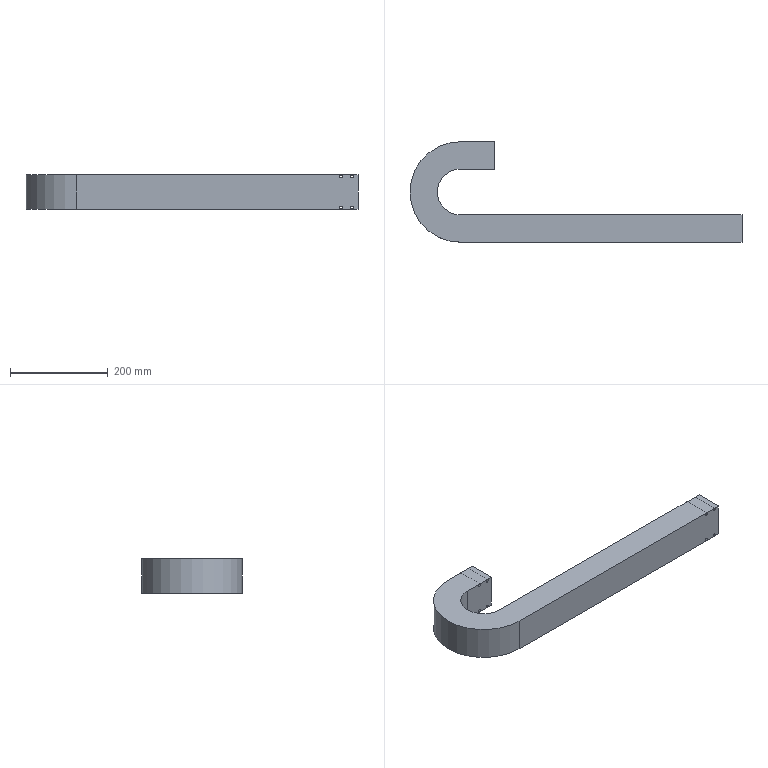Part | NX | 1 solid | 26 faces | box 681 x 206 x 70 mm | volume 1463808 mm3 | plane 14 | cylinder 12 | commonest cylinder face diameters 5.8 x8 94 x1 105 x1 195 x1 206 x1
STEP:
#1=CARTESIAN_POINT('',(0.,22.5,25.));
#2=VERTEX_POINT('',#1);
#3=CARTESIAN_POINT('',(0.,22.5,-25.));
#4=VERTEX_POINT('',#3);
#5=CARTESIAN_POINT('',(0.,22.5,25.));
#6=DIRECTION('',(0.,0.,-1.));
#7=VECTOR('',#6,1000.);
#8=LINE('',#5,#7);
#9=EDGE_CURVE('',#2,#4,#8,.T.);
#10=ORIENTED_EDGE('',*,*,#9,.T.);
#11=CARTESIAN_POINT('',(578.,22.5,-25.));
#12=VERTEX_POINT('',#11);
#13=CARTESIAN_POINT('',(0.,22.5,-25.));
#14=DIRECTION('',(1.,0.,0.));
#15=VECTOR('',#14,1000.);
#16=LINE('',#13,#15);
#17=EDGE_CURVE('',#4,#12,#16,.T.);
#18=ORIENTED_EDGE('',*,*,#17,.T.);
#19=CARTESIAN_POINT('',(578.,22.5,25.));
#20=VERTEX_POINT('',#19);
#21=CARTESIAN_POINT('',(578.,22.5,25.));
#22=DIRECTION('',(0.,0.,-1.));
#23=VECTOR('',#22,1000.);
#24=LINE('',#21,#23);
#25=EDGE_CURVE('',#20,#12,#24,.T.);
#26=ORIENTED_EDGE('',*,*,#25,.F.);
#27=CARTESIAN_POINT('',(0.,22.5,25.));
#28=DIRECTION('',(1.,0.,0.));
#29=VECTOR('',#28,1000.);
#30=LINE('',#27,#29);
#31=EDGE_CURVE('',#2,#20,#30,.T.);
#32=ORIENTED_EDGE('',*,*,#31,.F.);
#33=EDGE_LOOP('',(#10,#18,#26,#32));
#34=FACE_BOUND('',#33,.T.);
#35=CARTESIAN_POINT('',(0.,22.5,25.));
#36=DIRECTION('',(0.,-1.,0.));
#37=DIRECTION('',(0.,0.,-1.));
#38=AXIS2_PLACEMENT_3D('',#35,#36,#37);
#39=PLANE('',#38);
#40=ADVANCED_FACE('',(#34),#39,.T.);
#41=CARTESIAN_POINT('',(0.,-22.5,-25.));
#42=VERTEX_POINT('',#41);
#43=CARTESIAN_POINT('',(0.,-22.5,25.));
#44=VERTEX_POINT('',#43);
#45=CARTESIAN_POINT('',(0.,-22.5,25.));
#46=DIRECTION('',(0.,0.,1.));
#47=VECTOR('',#46,1000.);
#48=LINE('',#45,#47);
#49=EDGE_CURVE('',#42,#44,#48,.T.);
#50=ORIENTED_EDGE('',*,*,#49,.T.);
#51=CARTESIAN_POINT('',(578.,-22.5,25.));
#52=VERTEX_POINT('',#51);
#53=CARTESIAN_POINT('',(0.,-22.5,25.));
#54=DIRECTION('',(1.,0.,0.));
#55=VECTOR('',#54,1000.);
#56=LINE('',#53,#55);
#57=EDGE_CURVE('',#44,#52,#56,.T.);
#58=ORIENTED_EDGE('',*,*,#57,.T.);
#59=CARTESIAN_POINT('',(578.,-22.5,-25.));
#60=VERTEX_POINT('',#59);
#61=CARTESIAN_POINT('',(578.,-22.5,25.));
#62=DIRECTION('',(0.,0.,1.));
#63=VECTOR('',#62,1000.);
#64=LINE('',#61,#63);
#65=EDGE_CURVE('',#60,#52,#64,.T.);
#66=ORIENTED_EDGE('',*,*,#65,.F.);
#67=CARTESIAN_POINT('',(0.,-22.5,-25.));
#68=DIRECTION('',(1.,0.,0.));
#69=VECTOR('',#68,1000.);
#70=LINE('',#67,#69);
#71=EDGE_CURVE('',#42,#60,#70,.T.);
#72=ORIENTED_EDGE('',*,*,#71,.F.);
#73=EDGE_LOOP('',(#50,#58,#66,#72));
#74=FACE_BOUND('',#73,.T.);
#75=CARTESIAN_POINT('',(0.,-22.5,25.));
#76=DIRECTION('',(0.,1.,0.));
#77=DIRECTION('',(0.,0.,1.));
#78=AXIS2_PLACEMENT_3D('',#75,#76,#77);
#79=PLANE('',#78);
#80=ADVANCED_FACE('',(#74),#79,.T.);
#81=CARTESIAN_POINT('',(543.,28.,34.9));
#82=VERTEX_POINT('',#81);
#83=CARTESIAN_POINT('',(543.,28.,32.));
#84=DIRECTION('',(0.,1.,0.));
#85=DIRECTION('',(0.,0.,1.));
#86=AXIS2_PLACEMENT_3D('',#83,#84,#85);
#87=CIRCLE('',#86,2.9);
#88=EDGE_CURVE('',#82,#82,#87,.T.);
#89=ORIENTED_EDGE('',*,*,#88,.F.);
#90=EDGE_LOOP('',(#89));
#91=FACE_BOUND('',#90,.T.);
#92=CARTESIAN_POINT('',(543.,28.,-29.1));
#93=VERTEX_POINT('',#92);
#94=CARTESIAN_POINT('',(543.,28.,-32.));
#95=DIRECTION('',(0.,1.,0.));
#96=DIRECTION('',(0.,0.,1.));
#97=AXIS2_PLACEMENT_3D('',#94,#95,#96);
#98=CIRCLE('',#97,2.9);
#99=EDGE_CURVE('',#93,#93,#98,.T.);
#100=ORIENTED_EDGE('',*,*,#99,.F.);
#101=EDGE_LOOP('',(#100));
#102=FACE_BOUND('',#101,.T.);
#103=CARTESIAN_POINT('',(565.5,28.,29.1));
#104=VERTEX_POINT('',#103);
#105=CARTESIAN_POINT('',(565.5,28.,32.));
#106=DIRECTION('',(0.,1.,0.));
#107=DIRECTION('',(0.,0.,-1.));
#108=AXIS2_PLACEMENT_3D('',#105,#106,#107);
#109=CIRCLE('',#108,2.9);
#110=EDGE_CURVE('',#104,#104,#109,.T.);
#111=ORIENTED_EDGE('',*,*,#110,.F.);
#112=EDGE_LOOP('',(#111));
#113=FACE_BOUND('',#112,.T.);
#114=CARTESIAN_POINT('',(565.5,28.,-29.1));
#115=VERTEX_POINT('',#114);
#116=CARTESIAN_POINT('',(565.5,28.,-32.));
#117=DIRECTION('',(0.,1.,0.));
#118=DIRECTION('',(0.,0.,1.));
#119=AXIS2_PLACEMENT_3D('',#116,#117,#118);
#120=CIRCLE('',#119,2.9);
#121=EDGE_CURVE('',#115,#115,#120,.T.);
#122=ORIENTED_EDGE('',*,*,#121,.F.);
#123=EDGE_LOOP('',(#122));
#124=FACE_BOUND('',#123,.T.);
#125=CARTESIAN_POINT('',(0.,28.,35.));
#126=VERTEX_POINT('',#125);
#127=CARTESIAN_POINT('',(0.,28.,-35.));
#128=VERTEX_POINT('',#127);
#129=CARTESIAN_POINT('',(0.,28.,35.));
#130=DIRECTION('',(0.,0.,-1.));
#131=VECTOR('',#130,1000.);
#132=LINE('',#129,#131);
#133=EDGE_CURVE('',#126,#128,#132,.T.);
#134=ORIENTED_EDGE('',*,*,#133,.F.);
#135=CARTESIAN_POINT('',(578.,28.,35.));
#136=VERTEX_POINT('',#135);
#137=CARTESIAN_POINT('',(0.,28.,35.));
#138=DIRECTION('',(1.,0.,0.));
#139=VECTOR('',#138,1000.);
#140=LINE('',#137,#139);
#141=EDGE_CURVE('',#126,#136,#140,.T.);
#142=ORIENTED_EDGE('',*,*,#141,.T.);
#143=CARTESIAN_POINT('',(578.,28.,-35.));
#144=VERTEX_POINT('',#143);
#145=CARTESIAN_POINT('',(578.,28.,35.));
#146=DIRECTION('',(0.,0.,-1.));
#147=VECTOR('',#146,1000.);
#148=LINE('',#145,#147);
#149=EDGE_CURVE('',#136,#144,#148,.T.);
#150=ORIENTED_EDGE('',*,*,#149,.T.);
#151=CARTESIAN_POINT('',(0.,28.,-35.));
#152=DIRECTION('',(1.,0.,0.));
#153=VECTOR('',#152,1000.);
#154=LINE('',#151,#153);
#155=EDGE_CURVE('',#128,#144,#154,.T.);
#156=ORIENTED_EDGE('',*,*,#155,.F.);
#157=EDGE_LOOP('',(#134,#142,#150,#156));
#158=FACE_BOUND('',#157,.T.);
#159=CARTESIAN_POINT('',(0.,28.,35.));
#160=DIRECTION('',(0.,-1.,0.));
#161=DIRECTION('',(0.,0.,-1.));
#162=AXIS2_PLACEMENT_3D('',#159,#160,#161);
#163=PLANE('',#162);
#164=ADVANCED_FACE('',(#91,#102,#113,#124,#158),#163,.F.);
#165=CARTESIAN_POINT('',(543.,-28.,34.9));
#166=VERTEX_POINT('',#165);
#167=CARTESIAN_POINT('',(543.,-28.,32.));
#168=DIRECTION('',(0.,1.,0.));
#169=DIRECTION('',(0.,0.,1.));
#170=AXIS2_PLACEMENT_3D('',#167,#168,#169);
#171=CIRCLE('',#170,2.9);
#172=EDGE_CURVE('',#166,#166,#171,.T.);
#173=ORIENTED_EDGE('',*,*,#172,.T.);
#174=EDGE_LOOP('',(#173));
#175=FACE_BOUND('',#174,.T.);
#176=CARTESIAN_POINT('',(543.,-28.,-29.1));
#177=VERTEX_POINT('',#176);
#178=CARTESIAN_POINT('',(543.,-28.,-32.));
#179=DIRECTION('',(0.,1.,0.));
#180=DIRECTION('',(0.,0.,1.));
#181=AXIS2_PLACEMENT_3D('',#178,#179,#180);
#182=CIRCLE('',#181,2.9);
#183=EDGE_CURVE('',#177,#177,#182,.T.);
#184=ORIENTED_EDGE('',*,*,#183,.T.);
#185=EDGE_LOOP('',(#184));
#186=FACE_BOUND('',#185,.T.);
#187=CARTESIAN_POINT('',(565.5,-28.,34.9));
#188=VERTEX_POINT('',#187);
#189=CARTESIAN_POINT('',(565.5,-28.,32.));
#190=DIRECTION('',(0.,1.,0.));
#191=DIRECTION('',(0.,0.,1.));
#192=AXIS2_PLACEMENT_3D('',#189,#190,#191);
#193=CIRCLE('',#192,2.9);
#194=EDGE_CURVE('',#188,#188,#193,.T.);
#195=ORIENTED_EDGE('',*,*,#194,.T.);
#196=EDGE_LOOP('',(#195));
#197=FACE_BOUND('',#196,.T.);
#198=CARTESIAN_POINT('',(565.5,-28.,-29.1));
#199=VERTEX_POINT('',#198);
#200=CARTESIAN_POINT('',(565.5,-28.,-32.));
#201=DIRECTION('',(0.,1.,0.));
#202=DIRECTION('',(0.,0.,1.));
#203=AXIS2_PLACEMENT_3D('',#200,#201,#202);
#204=CIRCLE('',#203,2.9);
#205=EDGE_CURVE('',#199,#199,#204,.T.);
#206=ORIENTED_EDGE('',*,*,#205,.T.);
#207=EDGE_LOOP('',(#206));
#208=FACE_BOUND('',#207,.T.);
#209=CARTESIAN_POINT('',(0.,-28.,-35.));
#210=VERTEX_POINT('',#209);
#211=CARTESIAN_POINT('',(0.,-28.,35.));
#212=VERTEX_POINT('',#211);
#213=CARTESIAN_POINT('',(0.,-28.,35.));
#214=DIRECTION('',(0.,0.,1.));
#215=VECTOR('',#214,1000.);
#216=LINE('',#213,#215);
#217=EDGE_CURVE('',#210,#212,#216,.T.);
#218=ORIENTED_EDGE('',*,*,#217,.F.);
#219=CARTESIAN_POINT('',(578.,-28.,-35.));
#220=VERTEX_POINT('',#219);
#221=CARTESIAN_POINT('',(0.,-28.,-35.));
#222=DIRECTION('',(1.,0.,0.));
#223=VECTOR('',#222,1000.);
#224=LINE('',#221,#223);
#225=EDGE_CURVE('',#210,#220,#224,.T.);
#226=ORIENTED_EDGE('',*,*,#225,.T.);
#227=CARTESIAN_POINT('',(578.,-28.,35.));
#228=VERTEX_POINT('',#227);
#229=CARTESIAN_POINT('',(578.,-28.,35.));
#230=DIRECTION('',(0.,0.,1.));
#231=VECTOR('',#230,1000.);
#232=LINE('',#229,#231);
#233=EDGE_CURVE('',#220,#228,#232,.T.);
#234=ORIENTED_EDGE('',*,*,#233,.T.);
#235=CARTESIAN_POINT('',(0.,-28.,35.));
#236=DIRECTION('',(1.,0.,0.));
#237=VECTOR('',#236,1000.);
#238=LINE('',#235,#237);
#239=EDGE_CURVE('',#212,#228,#238,.T.);
#240=ORIENTED_EDGE('',*,*,#239,.F.);
#241=EDGE_LOOP('',(#218,#226,#234,#240));
#242=FACE_BOUND('',#241,.T.);
#243=CARTESIAN_POINT('',(0.,-28.,35.));
#244=DIRECTION('',(0.,1.,0.));
#245=DIRECTION('',(0.,0.,1.));
#246=AXIS2_PLACEMENT_3D('',#243,#244,#245);
#247=PLANE('',#246);
#248=ADVANCED_FACE('',(#175,#186,#197,#208,#242),#247,.F.);
#249=CARTESIAN_POINT('',(0.,127.5,25.));
#250=VERTEX_POINT('',#249);
#251=CARTESIAN_POINT('',(0.,127.5,-25.));
#252=VERTEX_POINT('',#251);
#253=CARTESIAN_POINT('',(0.,127.5,25.));
#254=DIRECTION('',(0.,0.,-1.));
#255=VECTOR('',#254,1000.);
#256=LINE('',#253,#255);
#257=EDGE_CURVE('',#250,#252,#256,.T.);
#258=ORIENTED_EDGE('',*,*,#257,.T.);
#259=CARTESIAN_POINT('',(0.,75.,-25.));
#260=DIRECTION('',(0.,0.,1.));
#261=DIRECTION('',(1.,0.,0.));
#262=AXIS2_PLACEMENT_3D('',#259,#260,#261);
#263=CIRCLE('',#262,52.5);
#264=EDGE_CURVE('',#252,#4,#263,.T.);
#265=ORIENTED_EDGE('',*,*,#264,.T.);
#266=ORIENTED_EDGE('',*,*,#9,.F.);
#267=CARTESIAN_POINT('',(0.,75.,25.));
#268=DIRECTION('',(0.,0.,1.));
#269=DIRECTION('',(1.,0.,0.));
#270=AXIS2_PLACEMENT_3D('',#267,#268,#269);
#271=CIRCLE('',#270,52.5);
#272=EDGE_CURVE('',#250,#2,#271,.T.);
#273=ORIENTED_EDGE('',*,*,#272,.F.);
#274=EDGE_LOOP('',(#258,#265,#266,#273));
#275=FACE_BOUND('',#274,.T.);
#276=CARTESIAN_POINT('',(0.,75.,0.));
#277=DIRECTION('',(0.,0.,1.));
#278=DIRECTION('',(1.,0.,0.));
#279=AXIS2_PLACEMENT_3D('',#276,#277,#278);
#280=CYLINDRICAL_SURFACE('',#279,52.5);
#281=ADVANCED_FACE('',(#275),#280,.T.);
#282=CARTESIAN_POINT('',(0.,172.5,-25.));
#283=VERTEX_POINT('',#282);
#284=CARTESIAN_POINT('',(0.,172.5,25.));
#285=VERTEX_POINT('',#284);
#286=CARTESIAN_POINT('',(0.,172.5,25.));
#287=DIRECTION('',(0.,0.,1.));
#288=VECTOR('',#287,1000.);
#289=LINE('',#286,#288);
#290=EDGE_CURVE('',#283,#285,#289,.T.);
#291=ORIENTED_EDGE('',*,*,#290,.T.);
#292=CARTESIAN_POINT('',(0.,75.,25.));
#293=DIRECTION('',(0.,0.,1.));
#294=DIRECTION('',(1.,0.,0.));
#295=AXIS2_PLACEMENT_3D('',#292,#293,#294);
#296=CIRCLE('',#295,97.5);
#297=EDGE_CURVE('',#285,#44,#296,.T.);
#298=ORIENTED_EDGE('',*,*,#297,.T.);
#299=ORIENTED_EDGE('',*,*,#49,.F.);
#300=CARTESIAN_POINT('',(0.,75.,-25.));
#301=DIRECTION('',(0.,0.,1.));
#302=DIRECTION('',(1.,0.,0.));
#303=AXIS2_PLACEMENT_3D('',#300,#301,#302);
#304=CIRCLE('',#303,97.5);
#305=EDGE_CURVE('',#283,#42,#304,.T.);
#306=ORIENTED_EDGE('',*,*,#305,.F.);
#307=EDGE_LOOP('',(#291,#298,#299,#306));
#308=FACE_BOUND('',#307,.T.);
#309=CARTESIAN_POINT('',(0.,75.,0.));
#310=DIRECTION('',(0.,0.,1.));
#311=DIRECTION('',(1.,0.,0.));
#312=AXIS2_PLACEMENT_3D('',#309,#310,#311);
#313=CYLINDRICAL_SURFACE('',#312,97.5);
#314=ADVANCED_FACE('',(#308),#313,.F.);
#315=CARTESIAN_POINT('',(0.,122.,35.));
#316=VERTEX_POINT('',#315);
#317=CARTESIAN_POINT('',(0.,122.,-35.));
#318=VERTEX_POINT('',#317);
#319=CARTESIAN_POINT('',(0.,122.,35.));
#320=DIRECTION('',(0.,0.,-1.));
#321=VECTOR('',#320,1000.);
#322=LINE('',#319,#321);
#323=EDGE_CURVE('',#316,#318,#322,.T.);
#324=ORIENTED_EDGE('',*,*,#323,.F.);
#325=CARTESIAN_POINT('',(0.,75.,35.));
#326=DIRECTION('',(0.,0.,1.));
#327=DIRECTION('',(1.,0.,0.));
#328=AXIS2_PLACEMENT_3D('',#325,#326,#327);
#329=CIRCLE('',#328,47.);
#330=EDGE_CURVE('',#316,#126,#329,.T.);
#331=ORIENTED_EDGE('',*,*,#330,.T.);
#332=ORIENTED_EDGE('',*,*,#133,.T.);
#333=CARTESIAN_POINT('',(0.,75.,-35.));
#334=DIRECTION('',(0.,0.,1.));
#335=DIRECTION('',(1.,0.,0.));
#336=AXIS2_PLACEMENT_3D('',#333,#334,#335);
#337=CIRCLE('',#336,47.);
#338=EDGE_CURVE('',#318,#128,#337,.T.);
#339=ORIENTED_EDGE('',*,*,#338,.F.);
#340=EDGE_LOOP('',(#324,#331,#332,#339));
#341=FACE_BOUND('',#340,.T.);
#342=CARTESIAN_POINT('',(0.,75.,0.));
#343=DIRECTION('',(0.,0.,1.));
#344=DIRECTION('',(1.,0.,0.));
#345=AXIS2_PLACEMENT_3D('',#342,#343,#344);
#346=CYLINDRICAL_SURFACE('',#345,47.);
#347=ADVANCED_FACE('',(#341),#346,.F.);
#348=CARTESIAN_POINT('',(0.,178.,-35.));
#349=VERTEX_POINT('',#348);
#350=CARTESIAN_POINT('',(0.,178.,35.));
#351=VERTEX_POINT('',#350);
#352=CARTESIAN_POINT('',(0.,178.,35.));
#353=DIRECTION('',(0.,0.,1.));
#354=VECTOR('',#353,1000.);
#355=LINE('',#352,#354);
#356=EDGE_CURVE('',#349,#351,#355,.T.);
#357=ORIENTED_EDGE('',*,*,#356,.F.);
#358=CARTESIAN_POINT('',(0.,75.,-35.));
#359=DIRECTION('',(0.,0.,1.));
#360=DIRECTION('',(1.,0.,0.));
#361=AXIS2_PLACEMENT_3D('',#358,#359,#360);
#362=CIRCLE('',#361,103.);
#363=EDGE_CURVE('',#349,#210,#362,.T.);
#364=ORIENTED_EDGE('',*,*,#363,.T.);
#365=ORIENTED_EDGE('',*,*,#217,.T.);
#366=CARTESIAN_POINT('',(0.,75.,35.));
#367=DIRECTION('',(0.,0.,1.));
#368=DIRECTION('',(1.,0.,0.));
#369=AXIS2_PLACEMENT_3D('',#366,#367,#368);
#370=CIRCLE('',#369,103.);
#371=EDGE_CURVE('',#351,#212,#370,.T.);
#372=ORIENTED_EDGE('',*,*,#371,.F.);
#373=EDGE_LOOP('',(#357,#364,#365,#372));
#374=FACE_BOUND('',#373,.T.);
#375=CARTESIAN_POINT('',(0.,75.,0.));
#376=DIRECTION('',(0.,0.,1.));
#377=DIRECTION('',(1.,0.,0.));
#378=AXIS2_PLACEMENT_3D('',#375,#376,#377);
#379=CYLINDRICAL_SURFACE('',#378,103.);
#380=ADVANCED_FACE('',(#374),#379,.T.);
#381=CARTESIAN_POINT('',(70.,172.5,25.));
#382=VERTEX_POINT('',#381);
#383=CARTESIAN_POINT('',(70.,127.5,25.));
#384=VERTEX_POINT('',#383);
#385=CARTESIAN_POINT('',(70.,127.5,25.));
#386=DIRECTION('',(0.,-1.,0.));
#387=VECTOR('',#386,1000.);
#388=LINE('',#385,#387);
#389=EDGE_CURVE('',#382,#384,#388,.T.);
#390=ORIENTED_EDGE('',*,*,#389,.T.);
#391=CARTESIAN_POINT('',(0.,127.5,25.));
#392=DIRECTION('',(1.,0.,0.));
#393=VECTOR('',#392,1000.);
#394=LINE('',#391,#393);
#395=EDGE_CURVE('',#250,#384,#394,.T.);
#396=ORIENTED_EDGE('',*,*,#395,.F.);
#397=ORIENTED_EDGE('',*,*,#272,.T.);
#398=ORIENTED_EDGE('',*,*,#31,.T.);
#399=CARTESIAN_POINT('',(578.,22.5,25.));
#400=DIRECTION('',(0.,1.,0.));
#401=VECTOR('',#400,1000.);
#402=LINE('',#399,#401);
#403=EDGE_CURVE('',#52,#20,#402,.T.);
#404=ORIENTED_EDGE('',*,*,#403,.F.);
#405=ORIENTED_EDGE('',*,*,#57,.F.);
#406=ORIENTED_EDGE('',*,*,#297,.F.);
#407=CARTESIAN_POINT('',(0.,172.5,25.));
#408=DIRECTION('',(1.,0.,0.));
#409=VECTOR('',#408,1000.);
#410=LINE('',#407,#409);
#411=EDGE_CURVE('',#285,#382,#410,.T.);
#412=ORIENTED_EDGE('',*,*,#411,.T.);
#413=EDGE_LOOP('',(#390,#396,#397,#398,#404,#405,#406,#412));
#414=FACE_BOUND('',#413,.T.);
#415=CARTESIAN_POINT('',(0.,127.5,25.));
#416=DIRECTION('',(0.,0.,1.));
#417=DIRECTION('',(0.,-1.,0.));
#418=AXIS2_PLACEMENT_3D('',#415,#416,#417);
#419=PLANE('',#418);
#420=ADVANCED_FACE('',(#414),#419,.F.);
#421=CARTESIAN_POINT('',(70.,127.5,-25.));
#422=VERTEX_POINT('',#421);
#423=CARTESIAN_POINT('',(70.,127.5,25.));
#424=DIRECTION('',(0.,0.,-1.));
#425=VECTOR('',#424,1000.);
#426=LINE('',#423,#425);
#427=EDGE_CURVE('',#384,#422,#426,.T.);
#428=ORIENTED_EDGE('',*,*,#427,.T.);
#429=CARTESIAN_POINT('',(0.,127.5,-25.));
#430=DIRECTION('',(1.,0.,0.));
#431=VECTOR('',#430,1000.);
#432=LINE('',#429,#431);
#433=EDGE_CURVE('',#252,#422,#432,.T.);
#434=ORIENTED_EDGE('',*,*,#433,.F.);
#435=ORIENTED_EDGE('',*,*,#257,.F.);
#436=ORIENTED_EDGE('',*,*,#395,.T.);
#437=EDGE_LOOP('',(#428,#434,#435,#436));
#438=FACE_BOUND('',#437,.T.);
#439=CARTESIAN_POINT('',(0.,127.5,25.));
#440=DIRECTION('',(0.,-1.,0.));
#441=DIRECTION('',(1.,0.,0.));
#442=AXIS2_PLACEMENT_3D('',#439,#440,#441);
#443=PLANE('',#442);
#444=ADVANCED_FACE('',(#438),#443,.F.);
#445=CARTESIAN_POINT('',(70.,172.5,-25.));
#446=VERTEX_POINT('',#445);
#447=CARTESIAN_POINT('',(70.,127.5,-25.));
#448=DIRECTION('',(0.,1.,0.));
#449=VECTOR('',#448,1000.);
#450=LINE('',#447,#449);
#451=EDGE_CURVE('',#422,#446,#450,.T.);
#452=ORIENTED_EDGE('',*,*,#451,.T.);
#453=CARTESIAN_POINT('',(0.,172.5,-25.));
#454=DIRECTION('',(1.,0.,0.));
#455=VECTOR('',#454,1000.);
#456=LINE('',#453,#455);
#457=EDGE_CURVE('',#283,#446,#456,.T.);
#458=ORIENTED_EDGE('',*,*,#457,.F.);
#459=ORIENTED_EDGE('',*,*,#305,.T.);
#460=ORIENTED_EDGE('',*,*,#71,.T.);
#461=CARTESIAN_POINT('',(578.,22.5,-25.));
#462=DIRECTION('',(0.,-1.,0.));
#463=VECTOR('',#462,1000.);
#464=LINE('',#461,#463);
#465=EDGE_CURVE('',#12,#60,#464,.T.);
#466=ORIENTED_EDGE('',*,*,#465,.F.);
#467=ORIENTED_EDGE('',*,*,#17,.F.);
#468=ORIENTED_EDGE('',*,*,#264,.F.);
#469=ORIENTED_EDGE('',*,*,#433,.T.);
#470=EDGE_LOOP('',(#452,#458,#459,#460,#466,#467,#468,#469));
#471=FACE_BOUND('',#470,.T.);
#472=CARTESIAN_POINT('',(0.,127.5,-25.));
#473=DIRECTION('',(0.,0.,-1.));
#474=DIRECTION('',(-1.,0.,0.));
#475=AXIS2_PLACEMENT_3D('',#472,#473,#474);
#476=PLANE('',#475);
#477=ADVANCED_FACE('',(#471),#476,.F.);
#478=CARTESIAN_POINT('',(70.,122.,-35.));
#479=VERTEX_POINT('',#478);
#480=CARTESIAN_POINT('',(70.,178.,-35.));
#481=VERTEX_POINT('',#480);
#482=CARTESIAN_POINT('',(70.,122.,-35.));
#483=DIRECTION('',(0.,1.,0.));
#484=VECTOR('',#483,1000.);
#485=LINE('',#482,#484);
#486=EDGE_CURVE('',#479,#481,#485,.T.);
#487=ORIENTED_EDGE('',*,*,#486,.F.);
#488=CARTESIAN_POINT('',(0.,122.,-35.));
#489=DIRECTION('',(1.,0.,0.));
#490=VECTOR('',#489,1000.);
#491=LINE('',#488,#490);
#492=EDGE_CURVE('',#318,#479,#491,.T.);
#493=ORIENTED_EDGE('',*,*,#492,.F.);
#494=ORIENTED_EDGE('',*,*,#338,.T.);
#495=ORIENTED_EDGE('',*,*,#155,.T.);
#496=CARTESIAN_POINT('',(578.,28.,-35.));
#497=DIRECTION('',(0.,-1.,0.));
#498=VECTOR('',#497,1000.);
#499=LINE('',#496,#498);
#500=EDGE_CURVE('',#144,#220,#499,.T.);
#501=ORIENTED_EDGE('',*,*,#500,.T.);
#502=ORIENTED_EDGE('',*,*,#225,.F.);
#503=ORIENTED_EDGE('',*,*,#363,.F.);
#504=CARTESIAN_POINT('',(0.,178.,-35.));
#505=DIRECTION('',(1.,0.,0.));
#506=VECTOR('',#505,1000.);
#507=LINE('',#504,#506);
#508=EDGE_CURVE('',#349,#481,#507,.T.);
#509=ORIENTED_EDGE('',*,*,#508,.T.);
#510=EDGE_LOOP('',(#487,#493,#494,#495,#501,#502,#503,#509));
#511=FACE_BOUND('',#510,.T.);
#512=CARTESIAN_POINT('',(0.,122.,-35.));
#513=DIRECTION('',(0.,0.,-1.));
#514=DIRECTION('',(-1.,0.,0.));
#515=AXIS2_PLACEMENT_3D('',#512,#513,#514);
#516=PLANE('',#515);
#517=ADVANCED_FACE('',(#511),#516,.T.);
#518=CARTESIAN_POINT('',(37.9,122.,32.));
#519=VERTEX_POINT('',#518);
#520=CARTESIAN_POINT('',(35.,122.,32.));
#521=DIRECTION('',(0.,-1.,0.));
#522=DIRECTION('',(1.,0.,0.));
#523=AXIS2_PLACEMENT_3D('',#520,#521,#522);
#524=CIRCLE('',#523,2.9);
#525=EDGE_CURVE('',#519,#519,#524,.T.);
#526=ORIENTED_EDGE('',*,*,#525,.F.);
#527=EDGE_LOOP('',(#526));
#528=FACE_BOUND('',#527,.T.);
#529=CARTESIAN_POINT('',(37.9,122.,-32.));
#530=VERTEX_POINT('',#529);
#531=CARTESIAN_POINT('',(35.,122.,-32.));
#532=DIRECTION('',(0.,-1.,0.));
#533=DIRECTION('',(1.,0.,0.));
#534=AXIS2_PLACEMENT_3D('',#531,#532,#533);
#535=CIRCLE('',#534,2.9);
#536=EDGE_CURVE('',#530,#530,#535,.T.);
#537=ORIENTED_EDGE('',*,*,#536,.F.);
#538=EDGE_LOOP('',(#537));
#539=FACE_BOUND('',#538,.T.);
#540=CARTESIAN_POINT('',(60.4,122.,32.));
#541=VERTEX_POINT('',#540);
#542=CARTESIAN_POINT('',(57.5,122.,32.));
#543=DIRECTION('',(0.,-1.,0.));
#544=DIRECTION('',(1.,0.,0.));
#545=AXIS2_PLACEMENT_3D('',#542,#543,#544);
#546=CIRCLE('',#545,2.9);
#547=EDGE_CURVE('',#541,#541,#546,.T.);
#548=ORIENTED_EDGE('',*,*,#547,.F.);
#549=EDGE_LOOP('',(#548));
#550=FACE_BOUND('',#549,.T.);
#551=CARTESIAN_POINT('',(60.4,122.,-32.));
#552=VERTEX_POINT('',#551);
#553=CARTESIAN_POINT('',(57.5,122.,-32.));
#554=DIRECTION('',(0.,-1.,0.));
#555=DIRECTION('',(1.,0.,0.));
#556=AXIS2_PLACEMENT_3D('',#553,#554,#555);
#557=CIRCLE('',#556,2.9);
#558=EDGE_CURVE('',#552,#552,#557,.T.);
#559=ORIENTED_EDGE('',*,*,#558,.F.);
#560=EDGE_LOOP('',(#559));
#561=FACE_BOUND('',#560,.T.);
#562=CARTESIAN_POINT('',(70.,122.,35.));
#563=VERTEX_POINT('',#562);
#564=CARTESIAN_POINT('',(70.,122.,35.));
#565=DIRECTION('',(0.,0.,-1.));
#566=VECTOR('',#565,1000.);
#567=LINE('',#564,#566);
#568=EDGE_CURVE('',#563,#479,#567,.T.);
#569=ORIENTED_EDGE('',*,*,#568,.F.);
#570=CARTESIAN_POINT('',(0.,122.,35.));
#571=DIRECTION('',(1.,0.,0.));
#572=VECTOR('',#571,1000.);
#573=LINE('',#570,#572);
#574=EDGE_CURVE('',#316,#563,#573,.T.);
#575=ORIENTED_EDGE('',*,*,#574,.F.);
#576=ORIENTED_EDGE('',*,*,#323,.T.);
#577=ORIENTED_EDGE('',*,*,#492,.T.);
#578=EDGE_LOOP('',(#569,#575,#576,#577));
#579=FACE_BOUND('',#578,.T.);
#580=CARTESIAN_POINT('',(0.,122.,35.));
#581=DIRECTION('',(0.,-1.,0.));
#582=DIRECTION('',(1.,0.,0.));
#583=AXIS2_PLACEMENT_3D('',#580,#581,#582);
#584=PLANE('',#583);
#585=ADVANCED_FACE('',(#528,#539,#550,#561,#579),#584,.T.);
#586=CARTESIAN_POINT('',(70.,178.,35.));
#587=VERTEX_POINT('',#586);
#588=CARTESIAN_POINT('',(70.,122.,35.));
#589=DIRECTION('',(0.,-1.,0.));
#590=VECTOR('',#589,1000.);
#591=LINE('',#588,#590);
#592=EDGE_CURVE('',#587,#563,#591,.T.);
#593=ORIENTED_EDGE('',*,*,#592,.F.);
#594=CARTESIAN_POINT('',(0.,178.,35.));
#595=DIRECTION('',(1.,0.,0.));
#596=VECTOR('',#595,1000.);
#597=LINE('',#594,#596);
#598=EDGE_CURVE('',#351,#587,#597,.T.);
#599=ORIENTED_EDGE('',*,*,#598,.F.);
#600=ORIENTED_EDGE('',*,*,#371,.T.);
#601=ORIENTED_EDGE('',*,*,#239,.T.);
#602=CARTESIAN_POINT('',(578.,28.,35.));
#603=DIRECTION('',(0.,1.,0.));
#604=VECTOR('',#603,1000.);
#605=LINE('',#602,#604);
#606=EDGE_CURVE('',#228,#136,#605,.T.);
#607=ORIENTED_EDGE('',*,*,#606,.T.);
#608=ORIENTED_EDGE('',*,*,#141,.F.);
#609=ORIENTED_EDGE('',*,*,#330,.F.);
#610=ORIENTED_EDGE('',*,*,#574,.T.);
#611=EDGE_LOOP('',(#593,#599,#600,#601,#607,#608,#609,#610));
#612=FACE_BOUND('',#611,.T.);
#613=CARTESIAN_POINT('',(0.,122.,35.));
#614=DIRECTION('',(0.,0.,1.));
#615=DIRECTION('',(1.,0.,0.));
#616=AXIS2_PLACEMENT_3D('',#613,#614,#615);
#617=PLANE('',#616);
#618=ADVANCED_FACE('',(#612),#617,.T.);
#619=CARTESIAN_POINT('',(35.,178.,34.9));
#620=VERTEX_POINT('',#619);
#621=CARTESIAN_POINT('',(35.,178.,32.));
#622=DIRECTION('',(0.,1.,0.));
#623=DIRECTION('',(0.,0.,1.));
#624=AXIS2_PLACEMENT_3D('',#621,#622,#623);
#625=CIRCLE('',#624,2.9);
#626=EDGE_CURVE('',#620,#620,#625,.T.);
#627=ORIENTED_EDGE('',*,*,#626,.F.);
#628=EDGE_LOOP('',(#627));
#629=FACE_BOUND('',#628,.T.);
#630=CARTESIAN_POINT('',(35.,178.,-29.1));
#631=VERTEX_POINT('',#630);
#632=CARTESIAN_POINT('',(35.,178.,-32.));
#633=DIRECTION('',(0.,1.,0.));
#634=DIRECTION('',(0.,0.,1.));
#635=AXIS2_PLACEMENT_3D('',#632,#633,#634);
#636=CIRCLE('',#635,2.9);
#637=EDGE_CURVE('',#631,#631,#636,.T.);
#638=ORIENTED_EDGE('',*,*,#637,.F.);
#639=EDGE_LOOP('',(#638));
#640=FACE_BOUND('',#639,.T.);
#641=CARTESIAN_POINT('',(57.5,178.,34.9));
#642=VERTEX_POINT('',#641);
#643=CARTESIAN_POINT('',(57.5,178.,32.));
#644=DIRECTION('',(0.,1.,0.));
#645=DIRECTION('',(0.,0.,1.));
#646=AXIS2_PLACEMENT_3D('',#643,#644,#645);
#647=CIRCLE('',#646,2.9);
#648=EDGE_CURVE('',#642,#642,#647,.T.);
#649=ORIENTED_EDGE('',*,*,#648,.F.);
#650=EDGE_LOOP('',(#649));
#651=FACE_BOUND('',#650,.T.);
#652=CARTESIAN_POINT('',(57.5,178.,-29.1));
#653=VERTEX_POINT('',#652);
#654=CARTESIAN_POINT('',(57.5,178.,-32.));
#655=DIRECTION('',(0.,1.,0.));
#656=DIRECTION('',(0.,0.,1.));
#657=AXIS2_PLACEMENT_3D('',#654,#655,#656);
#658=CIRCLE('',#657,2.9);
#659=EDGE_CURVE('',#653,#653,#658,.T.);
#660=ORIENTED_EDGE('',*,*,#659,.F.);
#661=EDGE_LOOP('',(#660));
#662=FACE_BOUND('',#661,.T.);
#663=CARTESIAN_POINT('',(70.,178.,35.));
#664=DIRECTION('',(0.,0.,1.));
#665=VECTOR('',#664,1000.);
#666=LINE('',#663,#665);
#667=EDGE_CURVE('',#481,#587,#666,.T.);
#668=ORIENTED_EDGE('',*,*,#667,.F.);
#669=ORIENTED_EDGE('',*,*,#508,.F.);
#670=ORIENTED_EDGE('',*,*,#356,.T.);
#671=ORIENTED_EDGE('',*,*,#598,.T.);
#672=EDGE_LOOP('',(#668,#669,#670,#671));
#673=FACE_BOUND('',#672,.T.);
#674=CARTESIAN_POINT('',(0.,178.,35.));
#675=DIRECTION('',(0.,1.,0.));
#676=DIRECTION('',(-1.,0.,0.));
#677=AXIS2_PLACEMENT_3D('',#674,#675,#676);
#678=PLANE('',#677);
#679=ADVANCED_FACE('',(#629,#640,#651,#662,#673),#678,.T.);
#680=CARTESIAN_POINT('',(70.,172.5,25.));
#681=DIRECTION('',(0.,0.,1.));
#682=VECTOR('',#681,1000.);
#683=LINE('',#680,#682);
#684=EDGE_CURVE('',#446,#382,#683,.T.);
#685=ORIENTED_EDGE('',*,*,#684,.T.);
#686=ORIENTED_EDGE('',*,*,#411,.F.);
#687=ORIENTED_EDGE('',*,*,#290,.F.);
#688=ORIENTED_EDGE('',*,*,#457,.T.);
#689=EDGE_LOOP('',(#685,#686,#687,#688));
#690=FACE_BOUND('',#689,.T.);
#691=CARTESIAN_POINT('',(0.,172.5,25.));
#692=DIRECTION('',(0.,1.,0.));
#693=DIRECTION('',(-1.,0.,0.));
#694=AXIS2_PLACEMENT_3D('',#691,#692,#693);
#695=PLANE('',#694);
#696=ADVANCED_FACE('',(#690),#695,.F.);
#697=ORIENTED_EDGE('',*,*,#500,.F.);
#698=ORIENTED_EDGE('',*,*,#149,.F.);
#699=ORIENTED_EDGE('',*,*,#606,.F.);
#700=ORIENTED_EDGE('',*,*,#233,.F.);
#701=EDGE_LOOP('',(#697,#698,#699,#700));
#702=FACE_BOUND('',#701,.T.);
#703=ORIENTED_EDGE('',*,*,#403,.T.);
#704=ORIENTED_EDGE('',*,*,#25,.T.);
#705=ORIENTED_EDGE('',*,*,#465,.T.);
#706=ORIENTED_EDGE('',*,*,#65,.T.);
#707=EDGE_LOOP('',(#703,#704,#705,#706));
#708=FACE_BOUND('',#707,.T.);
#709=CARTESIAN_POINT('',(578.,150.,0.));
#710=DIRECTION('',(1.,0.,0.));
#711=DIRECTION('',(0.,0.,1.));
#712=AXIS2_PLACEMENT_3D('',#709,#710,#711);
#713=PLANE('',#712);
#714=ADVANCED_FACE('',(#702,#708),#713,.T.);
#715=ORIENTED_EDGE('',*,*,#486,.T.);
#716=ORIENTED_EDGE('',*,*,#667,.T.);
#717=ORIENTED_EDGE('',*,*,#592,.T.);
#718=ORIENTED_EDGE('',*,*,#568,.T.);
#719=EDGE_LOOP('',(#715,#716,#717,#718));
#720=FACE_BOUND('',#719,.T.);
#721=ORIENTED_EDGE('',*,*,#389,.F.);
#722=ORIENTED_EDGE('',*,*,#684,.F.);
#723=ORIENTED_EDGE('',*,*,#451,.F.);
#724=ORIENTED_EDGE('',*,*,#427,.F.);
#725=EDGE_LOOP('',(#721,#722,#723,#724));
#726=FACE_BOUND('',#725,.T.);
#727=CARTESIAN_POINT('',(70.,0.,0.));
#728=DIRECTION('',(-1.,0.,0.));
#729=DIRECTION('',(0.,0.,1.));
#730=AXIS2_PLACEMENT_3D('',#727,#728,#729);
#731=PLANE('',#730);
#732=ADVANCED_FACE('',(#720,#726),#731,.F.);
#733=ORIENTED_EDGE('',*,*,#558,.T.);
#734=EDGE_LOOP('',(#733));
#735=FACE_BOUND('',#734,.T.);
#736=ORIENTED_EDGE('',*,*,#659,.T.);
#737=EDGE_LOOP('',(#736));
#738=FACE_BOUND('',#737,.T.);
#739=CARTESIAN_POINT('',(57.5,78.,-32.));
#740=DIRECTION('',(0.,1.,0.));
#741=DIRECTION('',(0.,0.,1.));
#742=AXIS2_PLACEMENT_3D('',#739,#740,#741);
#743=CYLINDRICAL_SURFACE('',#742,2.9);
#744=ADVANCED_FACE('',(#735,#738),#743,.F.);
#745=ORIENTED_EDGE('',*,*,#547,.T.);
#746=EDGE_LOOP('',(#745));
#747=FACE_BOUND('',#746,.T.);
#748=ORIENTED_EDGE('',*,*,#648,.T.);
#749=EDGE_LOOP('',(#748));
#750=FACE_BOUND('',#749,.T.);
#751=CARTESIAN_POINT('',(57.5,78.,32.));
#752=DIRECTION('',(0.,1.,0.));
#753=DIRECTION('',(0.,0.,1.));
#754=AXIS2_PLACEMENT_3D('',#751,#752,#753);
#755=CYLINDRICAL_SURFACE('',#754,2.9);
#756=ADVANCED_FACE('',(#747,#750),#755,.F.);
#757=ORIENTED_EDGE('',*,*,#536,.T.);
#758=EDGE_LOOP('',(#757));
#759=FACE_BOUND('',#758,.T.);
#760=ORIENTED_EDGE('',*,*,#637,.T.);
#761=EDGE_LOOP('',(#760));
#762=FACE_BOUND('',#761,.T.);
#763=CARTESIAN_POINT('',(35.,78.,-32.));
#764=DIRECTION('',(0.,1.,0.));
#765=DIRECTION('',(0.,0.,1.));
#766=AXIS2_PLACEMENT_3D('',#763,#764,#765);
#767=CYLINDRICAL_SURFACE('',#766,2.9);
#768=ADVANCED_FACE('',(#759,#762),#767,.F.);
#769=ORIENTED_EDGE('',*,*,#525,.T.);
#770=EDGE_LOOP('',(#769));
#771=FACE_BOUND('',#770,.T.);
#772=ORIENTED_EDGE('',*,*,#626,.T.);
#773=EDGE_LOOP('',(#772));
#774=FACE_BOUND('',#773,.T.);
#775=CARTESIAN_POINT('',(35.,78.,32.));
#776=DIRECTION('',(0.,1.,0.));
#777=DIRECTION('',(0.,0.,1.));
#778=AXIS2_PLACEMENT_3D('',#775,#776,#777);
#779=CYLINDRICAL_SURFACE('',#778,2.9);
#780=ADVANCED_FACE('',(#771,#774),#779,.F.);
#781=ORIENTED_EDGE('',*,*,#121,.T.);
#782=EDGE_LOOP('',(#781));
#783=FACE_BOUND('',#782,.T.);
#784=ORIENTED_EDGE('',*,*,#205,.F.);
#785=EDGE_LOOP('',(#784));
#786=FACE_BOUND('',#785,.T.);
#787=CARTESIAN_POINT('',(565.5,-80.,-32.));
#788=DIRECTION('',(0.,1.,0.));
#789=DIRECTION('',(0.,0.,1.));
#790=AXIS2_PLACEMENT_3D('',#787,#788,#789);
#791=CYLINDRICAL_SURFACE('',#790,2.9);
#792=ADVANCED_FACE('',(#783,#786),#791,.F.);
#793=ORIENTED_EDGE('',*,*,#110,.T.);
#794=EDGE_LOOP('',(#793));
#795=FACE_BOUND('',#794,.T.);
#796=ORIENTED_EDGE('',*,*,#194,.F.);
#797=EDGE_LOOP('',(#796));
#798=FACE_BOUND('',#797,.T.);
#799=CARTESIAN_POINT('',(565.5,-80.,32.));
#800=DIRECTION('',(0.,1.,0.));
#801=DIRECTION('',(0.,0.,1.));
#802=AXIS2_PLACEMENT_3D('',#799,#800,#801);
#803=CYLINDRICAL_SURFACE('',#802,2.9);
#804=ADVANCED_FACE('',(#795,#798),#803,.F.);
#805=ORIENTED_EDGE('',*,*,#99,.T.);
#806=EDGE_LOOP('',(#805));
#807=FACE_BOUND('',#806,.T.);
#808=ORIENTED_EDGE('',*,*,#183,.F.);
#809=EDGE_LOOP('',(#808));
#810=FACE_BOUND('',#809,.T.);
#811=CARTESIAN_POINT('',(543.,-80.,-32.));
#812=DIRECTION('',(0.,1.,0.));
#813=DIRECTION('',(0.,0.,1.));
#814=AXIS2_PLACEMENT_3D('',#811,#812,#813);
#815=CYLINDRICAL_SURFACE('',#814,2.9);
#816=ADVANCED_FACE('',(#807,#810),#815,.F.);
#817=ORIENTED_EDGE('',*,*,#88,.T.);
#818=EDGE_LOOP('',(#817));
#819=FACE_BOUND('',#818,.T.);
#820=ORIENTED_EDGE('',*,*,#172,.F.);
#821=EDGE_LOOP('',(#820));
#822=FACE_BOUND('',#821,.T.);
#823=CARTESIAN_POINT('',(543.,-80.,32.));
#824=DIRECTION('',(0.,1.,0.));
#825=DIRECTION('',(0.,0.,1.));
#826=AXIS2_PLACEMENT_3D('',#823,#824,#825);
#827=CYLINDRICAL_SURFACE('',#826,2.9);
#828=ADVANCED_FACE('',(#819,#822),#827,.F.);
#829=CLOSED_SHELL('',(#40,#80,#164,#248,#281,#314,#347,#380,#420,#444,#477,#517,#585,#618,#679,#696,#714,#732,#744,#756,#768,#780,#792,#804,#816,#828));
#830=MANIFOLD_SOLID_BREP('',#829);
#831=(LENGTH_UNIT()NAMED_UNIT(*)SI_UNIT(.MILLI.,.METRE.));
#832=UNCERTAINTY_MEASURE_WITH_UNIT(LENGTH_MEASURE(0.00001),#831,'','');
#833=(NAMED_UNIT(*)PLANE_ANGLE_UNIT()SI_UNIT($,.RADIAN.));
#834=(NAMED_UNIT(*)SI_UNIT($,.STERADIAN.)SOLID_ANGLE_UNIT());
#835=(GEOMETRIC_REPRESENTATION_CONTEXT(3)GLOBAL_UNCERTAINTY_ASSIGNED_CONTEXT((#832))GLOBAL_UNIT_ASSIGNED_CONTEXT((#831,#833,#834))REPRESENTATION_CONTEXT('',''));
#836=ADVANCED_BREP_SHAPE_REPRESENTATION('',(#830),#835);